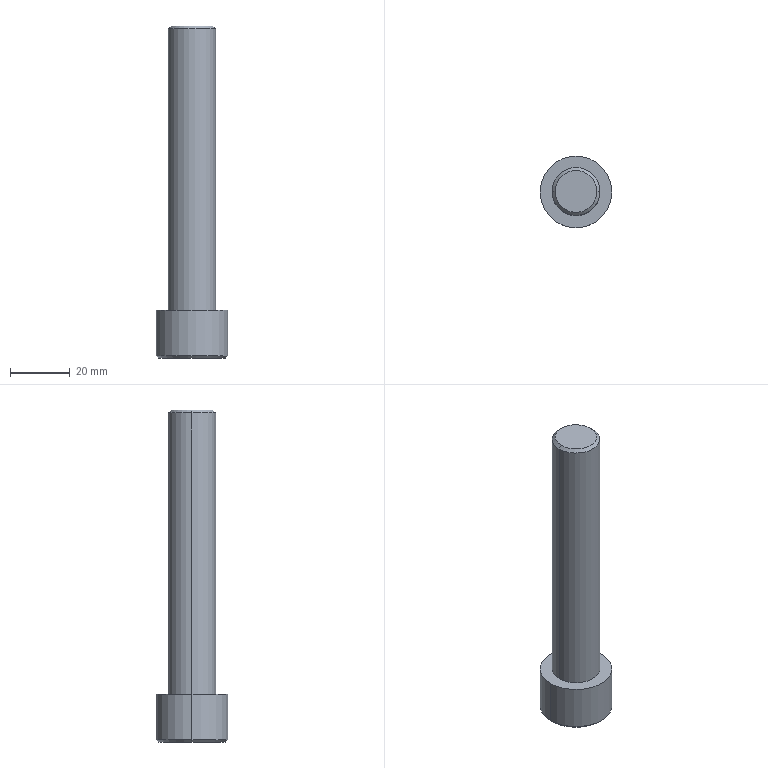Part | Creo | 1 solid | 18 faces | box 24 x 24 x 111 mm | volume 24662 mm3 | plane 10 | cylinder 4 | cone 4 | commonest cylinder face diameters 16 x2 24 x2
STEP:
#1=CARTESIAN_POINT('',(-139.,248.,-132.5));
#2=VERTEX_POINT('',#1);
#3=CARTESIAN_POINT('',(-115.,248.,-132.5));
#4=VERTEX_POINT('',#3);
#5=CARTESIAN_POINT('',(-127.,248.,-132.5));
#6=DIRECTION('',(0.,0.,1.));
#7=DIRECTION('',(-1.,0.,0.));
#8=AXIS2_PLACEMENT_3D('',#5,#6,#7);
#9=CIRCLE('',#8,12.);
#10=EDGE_CURVE('',#2,#4,#9,.T.);
#11=ORIENTED_EDGE('',*,*,#10,.F.);
#12=CARTESIAN_POINT('',(-127.,248.,-132.5));
#13=DIRECTION('',(0.,0.,1.));
#14=DIRECTION('',(1.,0.,0.));
#15=AXIS2_PLACEMENT_3D('',#12,#13,#14);
#16=CIRCLE('',#15,12.);
#17=EDGE_CURVE('',#4,#2,#16,.T.);
#18=ORIENTED_EDGE('',*,*,#17,.F.);
#19=EDGE_LOOP('',(#11,#18));
#20=FACE_OUTER_BOUND('',#19,.F.);
#21=CARTESIAN_POINT('',(-119.,248.,-132.5));
#22=VERTEX_POINT('',#21);
#23=CARTESIAN_POINT('',(-135.,248.,-132.5));
#24=VERTEX_POINT('',#23);
#25=CARTESIAN_POINT('',(-127.,248.,-132.5));
#26=DIRECTION('',(0.,0.,-1.));
#27=DIRECTION('',(1.,0.,0.));
#28=AXIS2_PLACEMENT_3D('',#25,#26,#27);
#29=CIRCLE('',#28,8.);
#30=EDGE_CURVE('',#22,#24,#29,.T.);
#31=ORIENTED_EDGE('',*,*,#30,.F.);
#32=CARTESIAN_POINT('',(-127.,248.,-132.5));
#33=DIRECTION('',(0.,0.,-1.));
#34=DIRECTION('',(-1.,0.,0.));
#35=AXIS2_PLACEMENT_3D('',#32,#33,#34);
#36=CIRCLE('',#35,8.);
#37=EDGE_CURVE('',#24,#22,#36,.T.);
#38=ORIENTED_EDGE('',*,*,#37,.F.);
#39=EDGE_LOOP('',(#31,#38));
#40=FACE_BOUND('',#39,.F.);
#41=CARTESIAN_POINT('',(-127.,248.,-132.5));
#42=DIRECTION('',(0.,0.,1.));
#43=DIRECTION('',(1.,0.,0.));
#44=AXIS2_PLACEMENT_3D('',#41,#42,#43);
#45=PLANE('',#44);
#46=ADVANCED_FACE('',(#20,#40),#45,.T.);
#47=CARTESIAN_POINT('',(-135.,248.,-38.5));
#48=VERTEX_POINT('',#47);
#49=CARTESIAN_POINT('',(-119.,248.,-38.5));
#50=VERTEX_POINT('',#49);
#51=CARTESIAN_POINT('',(-127.,248.,-38.5));
#52=DIRECTION('',(0.,0.,1.));
#53=DIRECTION('',(-1.,0.,0.));
#54=AXIS2_PLACEMENT_3D('',#51,#52,#53);
#55=CIRCLE('',#54,8.);
#56=EDGE_CURVE('',#48,#50,#55,.T.);
#57=ORIENTED_EDGE('',*,*,#56,.T.);
#58=CARTESIAN_POINT('',(-119.,248.,-132.5));
#59=DIRECTION('',(0.,0.,1.));
#60=VECTOR('',#59,94.);
#61=LINE('',#58,#60);
#62=EDGE_CURVE('',#22,#50,#61,.T.);
#63=ORIENTED_EDGE('',*,*,#62,.F.);
#64=ORIENTED_EDGE('',*,*,#30,.T.);
#65=CARTESIAN_POINT('',(-135.,248.,-132.5));
#66=DIRECTION('',(0.,0.,1.));
#67=VECTOR('',#66,94.);
#68=LINE('',#65,#67);
#69=EDGE_CURVE('',#24,#48,#68,.T.);
#70=ORIENTED_EDGE('',*,*,#69,.T.);
#71=EDGE_LOOP('',(#57,#63,#64,#70));
#72=FACE_OUTER_BOUND('',#71,.F.);
#73=CARTESIAN_POINT('',(-127.,248.,-150.5));
#74=DIRECTION('',(0.,0.,1.));
#75=DIRECTION('',(1.,0.,0.));
#76=AXIS2_PLACEMENT_3D('',#73,#74,#75);
#77=CYLINDRICAL_SURFACE('',#76,8.);
#78=ADVANCED_FACE('',(#72),#77,.T.);
#79=CARTESIAN_POINT('',(-134.,248.,-37.5));
#80=VERTEX_POINT('',#79);
#81=CARTESIAN_POINT('',(-120.,248.,-37.5));
#82=VERTEX_POINT('',#81);
#83=CARTESIAN_POINT('',(-127.,248.,-37.5));
#84=DIRECTION('',(0.,0.,1.));
#85=DIRECTION('',(-1.,0.,0.));
#86=AXIS2_PLACEMENT_3D('',#83,#84,#85);
#87=CIRCLE('',#86,7.);
#88=EDGE_CURVE('',#80,#82,#87,.T.);
#89=ORIENTED_EDGE('',*,*,#88,.T.);
#90=CARTESIAN_POINT('',(-120.,248.,-37.5));
#91=DIRECTION('',(0.7071,0.,-0.7071));
#92=VECTOR('',#91,1.414);
#93=LINE('',#90,#92);
#94=EDGE_CURVE('',#82,#50,#93,.T.);
#95=ORIENTED_EDGE('',*,*,#94,.T.);
#96=ORIENTED_EDGE('',*,*,#56,.F.);
#97=CARTESIAN_POINT('',(-134.,248.,-37.5));
#98=DIRECTION('',(-0.7071,0.,-0.7071));
#99=VECTOR('',#98,1.414);
#100=LINE('',#97,#99);
#101=EDGE_CURVE('',#80,#48,#100,.T.);
#102=ORIENTED_EDGE('',*,*,#101,.F.);
#103=EDGE_LOOP('',(#89,#95,#96,#102));
#104=FACE_OUTER_BOUND('',#103,.F.);
#105=CARTESIAN_POINT('',(-127.,248.,-38.));
#106=DIRECTION('',(0.,0.,-1.));
#107=DIRECTION('',(-1.,0.,0.));
#108=AXIS2_PLACEMENT_3D('',#105,#106,#107);
#109=CONICAL_SURFACE('',#108,7.5,45.);
#110=ADVANCED_FACE('',(#104),#109,.T.);
#111=CARTESIAN_POINT('',(-127.,248.,-37.5));
#112=DIRECTION('',(0.,0.,1.));
#113=DIRECTION('',(1.,0.,0.));
#114=AXIS2_PLACEMENT_3D('',#111,#112,#113);
#115=CIRCLE('',#114,7.);
#116=EDGE_CURVE('',#82,#80,#115,.T.);
#117=ORIENTED_EDGE('',*,*,#116,.F.);
#118=ORIENTED_EDGE('',*,*,#88,.F.);
#119=EDGE_LOOP('',(#117,#118));
#120=FACE_OUTER_BOUND('',#119,.F.);
#121=CARTESIAN_POINT('',(-127.,248.,-37.5));
#122=DIRECTION('',(0.,0.,1.));
#123=DIRECTION('',(1.,0.,0.));
#124=AXIS2_PLACEMENT_3D('',#121,#122,#123);
#125=PLANE('',#124);
#126=ADVANCED_FACE('',(#120),#125,.T.);
#127=ORIENTED_EDGE('',*,*,#116,.T.);
#128=ORIENTED_EDGE('',*,*,#101,.T.);
#129=CARTESIAN_POINT('',(-127.,248.,-38.5));
#130=DIRECTION('',(0.,0.,1.));
#131=DIRECTION('',(1.,0.,0.));
#132=AXIS2_PLACEMENT_3D('',#129,#130,#131);
#133=CIRCLE('',#132,8.);
#134=EDGE_CURVE('',#50,#48,#133,.T.);
#135=ORIENTED_EDGE('',*,*,#134,.F.);
#136=ORIENTED_EDGE('',*,*,#94,.F.);
#137=EDGE_LOOP('',(#127,#128,#135,#136));
#138=FACE_OUTER_BOUND('',#137,.F.);
#139=CARTESIAN_POINT('',(-127.,248.,-38.));
#140=DIRECTION('',(0.,0.,-1.));
#141=DIRECTION('',(-1.,0.,0.));
#142=AXIS2_PLACEMENT_3D('',#139,#140,#141);
#143=CONICAL_SURFACE('',#142,7.5,45.);
#144=ADVANCED_FACE('',(#138),#143,.T.);
#145=ORIENTED_EDGE('',*,*,#134,.T.);
#146=ORIENTED_EDGE('',*,*,#69,.F.);
#147=ORIENTED_EDGE('',*,*,#37,.T.);
#148=ORIENTED_EDGE('',*,*,#62,.T.);
#149=EDGE_LOOP('',(#145,#146,#147,#148));
#150=FACE_OUTER_BOUND('',#149,.F.);
#151=CARTESIAN_POINT('',(-127.,248.,-150.5));
#152=DIRECTION('',(0.,0.,1.));
#153=DIRECTION('',(1.,0.,0.));
#154=AXIS2_PLACEMENT_3D('',#151,#152,#153);
#155=CYLINDRICAL_SURFACE('',#154,8.);
#156=ADVANCED_FACE('',(#150),#155,.T.);
#157=CARTESIAN_POINT('',(-115.,248.,-147.7));
#158=VERTEX_POINT('',#157);
#159=CARTESIAN_POINT('',(-139.,248.,-147.7));
#160=VERTEX_POINT('',#159);
#161=CARTESIAN_POINT('',(-127.,248.,-147.7));
#162=DIRECTION('',(0.,0.,-1.));
#163=DIRECTION('',(1.,0.,0.));
#164=AXIS2_PLACEMENT_3D('',#161,#162,#163);
#165=CIRCLE('',#164,12.);
#166=EDGE_CURVE('',#158,#160,#165,.T.);
#167=ORIENTED_EDGE('',*,*,#166,.T.);
#168=CARTESIAN_POINT('',(-139.,248.,-147.7));
#169=DIRECTION('',(0.,0.,1.));
#170=VECTOR('',#169,15.2);
#171=LINE('',#168,#170);
#172=EDGE_CURVE('',#160,#2,#171,.T.);
#173=ORIENTED_EDGE('',*,*,#172,.T.);
#174=ORIENTED_EDGE('',*,*,#10,.T.);
#175=CARTESIAN_POINT('',(-115.,248.,-147.7));
#176=DIRECTION('',(0.,0.,1.));
#177=VECTOR('',#176,15.2);
#178=LINE('',#175,#177);
#179=EDGE_CURVE('',#158,#4,#178,.T.);
#180=ORIENTED_EDGE('',*,*,#179,.F.);
#181=EDGE_LOOP('',(#167,#173,#174,#180));
#182=FACE_OUTER_BOUND('',#181,.F.);
#183=CARTESIAN_POINT('',(-127.,248.,-150.5));
#184=DIRECTION('',(0.,0.,1.));
#185=DIRECTION('',(1.,0.,0.));
#186=AXIS2_PLACEMENT_3D('',#183,#184,#185);
#187=CYLINDRICAL_SURFACE('',#186,12.);
#188=ADVANCED_FACE('',(#182),#187,.T.);
#189=CARTESIAN_POINT('',(-115.8,248.,-148.5));
#190=VERTEX_POINT('',#189);
#191=CARTESIAN_POINT('',(-138.2,248.,-148.5));
#192=VERTEX_POINT('',#191);
#193=CARTESIAN_POINT('',(-127.,248.,-148.5));
#194=DIRECTION('',(0.,0.,-1.));
#195=DIRECTION('',(1.,0.,0.));
#196=AXIS2_PLACEMENT_3D('',#193,#194,#195);
#197=CIRCLE('',#196,11.2);
#198=EDGE_CURVE('',#190,#192,#197,.T.);
#199=ORIENTED_EDGE('',*,*,#198,.T.);
#200=CARTESIAN_POINT('',(-138.2,248.,-148.5));
#201=DIRECTION('',(-0.7071,0.,0.7071));
#202=VECTOR('',#201,1.131);
#203=LINE('',#200,#202);
#204=EDGE_CURVE('',#192,#160,#203,.T.);
#205=ORIENTED_EDGE('',*,*,#204,.T.);
#206=ORIENTED_EDGE('',*,*,#166,.F.);
#207=CARTESIAN_POINT('',(-115.8,248.,-148.5));
#208=DIRECTION('',(0.7071,0.,0.7071));
#209=VECTOR('',#208,1.131);
#210=LINE('',#207,#209);
#211=EDGE_CURVE('',#190,#158,#210,.T.);
#212=ORIENTED_EDGE('',*,*,#211,.F.);
#213=EDGE_LOOP('',(#199,#205,#206,#212));
#214=FACE_OUTER_BOUND('',#213,.F.);
#215=CARTESIAN_POINT('',(-127.,248.,-148.1));
#216=DIRECTION('',(0.,0.,1.));
#217=DIRECTION('',(1.,0.,0.));
#218=AXIS2_PLACEMENT_3D('',#215,#216,#217);
#219=CONICAL_SURFACE('',#218,11.6,45.);
#220=ADVANCED_FACE('',(#214),#219,.T.);
#221=ORIENTED_EDGE('',*,*,#198,.F.);
#222=CARTESIAN_POINT('',(-127.,248.,-148.5));
#223=DIRECTION('',(0.,0.,-1.));
#224=DIRECTION('',(-1.,0.,0.));
#225=AXIS2_PLACEMENT_3D('',#222,#223,#224);
#226=CIRCLE('',#225,11.2);
#227=EDGE_CURVE('',#192,#190,#226,.T.);
#228=ORIENTED_EDGE('',*,*,#227,.F.);
#229=EDGE_LOOP('',(#221,#228));
#230=FACE_OUTER_BOUND('',#229,.F.);
#231=CARTESIAN_POINT('',(-134.,243.959,-148.5));
#232=VERTEX_POINT('',#231);
#233=CARTESIAN_POINT('',(-127.,239.917,-148.5));
#234=VERTEX_POINT('',#233);
#235=CARTESIAN_POINT('',(-134.,243.959,-148.5));
#236=DIRECTION('',(0.866,-0.5,0.));
#237=VECTOR('',#236,8.083);
#238=LINE('',#235,#237);
#239=EDGE_CURVE('',#232,#234,#238,.T.);
#240=ORIENTED_EDGE('',*,*,#239,.F.);
#241=CARTESIAN_POINT('',(-134.,252.041,-148.5));
#242=VERTEX_POINT('',#241);
#243=CARTESIAN_POINT('',(-134.,252.041,-148.5));
#244=DIRECTION('',(0.,-1.,0.));
#245=VECTOR('',#244,8.083);
#246=LINE('',#243,#245);
#247=EDGE_CURVE('',#242,#232,#246,.T.);
#248=ORIENTED_EDGE('',*,*,#247,.F.);
#249=CARTESIAN_POINT('',(-127.,256.083,-148.5));
#250=VERTEX_POINT('',#249);
#251=CARTESIAN_POINT('',(-127.,256.083,-148.5));
#252=DIRECTION('',(-0.866,-0.5,0.));
#253=VECTOR('',#252,8.083);
#254=LINE('',#251,#253);
#255=EDGE_CURVE('',#250,#242,#254,.T.);
#256=ORIENTED_EDGE('',*,*,#255,.F.);
#257=CARTESIAN_POINT('',(-120.,252.041,-148.5));
#258=VERTEX_POINT('',#257);
#259=CARTESIAN_POINT('',(-120.,252.041,-148.5));
#260=DIRECTION('',(-0.866,0.5,0.));
#261=VECTOR('',#260,8.083);
#262=LINE('',#259,#261);
#263=EDGE_CURVE('',#258,#250,#262,.T.);
#264=ORIENTED_EDGE('',*,*,#263,.F.);
#265=CARTESIAN_POINT('',(-120.,243.959,-148.5));
#266=VERTEX_POINT('',#265);
#267=CARTESIAN_POINT('',(-120.,243.959,-148.5));
#268=DIRECTION('',(0.,1.,0.));
#269=VECTOR('',#268,8.083);
#270=LINE('',#267,#269);
#271=EDGE_CURVE('',#266,#258,#270,.T.);
#272=ORIENTED_EDGE('',*,*,#271,.F.);
#273=CARTESIAN_POINT('',(-127.,239.917,-148.5));
#274=DIRECTION('',(0.866,0.5,0.));
#275=VECTOR('',#274,8.083);
#276=LINE('',#273,#275);
#277=EDGE_CURVE('',#234,#266,#276,.T.);
#278=ORIENTED_EDGE('',*,*,#277,.F.);
#279=EDGE_LOOP('',(#240,#248,#256,#264,#272,#278));
#280=FACE_BOUND('',#279,.F.);
#281=CARTESIAN_POINT('',(-127.,248.,-148.5));
#282=DIRECTION('',(0.,0.,1.));
#283=DIRECTION('',(1.,0.,0.));
#284=AXIS2_PLACEMENT_3D('',#281,#282,#283);
#285=PLANE('',#284);
#286=ADVANCED_FACE('',(#230,#280),#285,.F.);
#287=ORIENTED_EDGE('',*,*,#227,.T.);
#288=ORIENTED_EDGE('',*,*,#211,.T.);
#289=CARTESIAN_POINT('',(-127.,248.,-147.7));
#290=DIRECTION('',(0.,0.,-1.));
#291=DIRECTION('',(-1.,0.,0.));
#292=AXIS2_PLACEMENT_3D('',#289,#290,#291);
#293=CIRCLE('',#292,12.);
#294=EDGE_CURVE('',#160,#158,#293,.T.);
#295=ORIENTED_EDGE('',*,*,#294,.F.);
#296=ORIENTED_EDGE('',*,*,#204,.F.);
#297=EDGE_LOOP('',(#287,#288,#295,#296));
#298=FACE_OUTER_BOUND('',#297,.F.);
#299=CARTESIAN_POINT('',(-127.,248.,-148.1));
#300=DIRECTION('',(0.,0.,1.));
#301=DIRECTION('',(1.,0.,0.));
#302=AXIS2_PLACEMENT_3D('',#299,#300,#301);
#303=CONICAL_SURFACE('',#302,11.6,45.);
#304=ADVANCED_FACE('',(#298),#303,.T.);
#305=ORIENTED_EDGE('',*,*,#294,.T.);
#306=ORIENTED_EDGE('',*,*,#179,.T.);
#307=ORIENTED_EDGE('',*,*,#17,.T.);
#308=ORIENTED_EDGE('',*,*,#172,.F.);
#309=EDGE_LOOP('',(#305,#306,#307,#308));
#310=FACE_OUTER_BOUND('',#309,.F.);
#311=CARTESIAN_POINT('',(-127.,248.,-150.5));
#312=DIRECTION('',(0.,0.,1.));
#313=DIRECTION('',(1.,0.,0.));
#314=AXIS2_PLACEMENT_3D('',#311,#312,#313);
#315=CYLINDRICAL_SURFACE('',#314,12.);
#316=ADVANCED_FACE('',(#310),#315,.T.);
#317=ORIENTED_EDGE('',*,*,#239,.T.);
#318=CARTESIAN_POINT('',(-127.,239.917,-138.9));
#319=VERTEX_POINT('',#318);
#320=CARTESIAN_POINT('',(-127.,239.917,-148.5));
#321=DIRECTION('',(0.,0.,1.));
#322=VECTOR('',#321,9.6);
#323=LINE('',#320,#322);
#324=EDGE_CURVE('',#234,#319,#323,.T.);
#325=ORIENTED_EDGE('',*,*,#324,.T.);
#326=CARTESIAN_POINT('',(-134.,243.959,-138.9));
#327=VERTEX_POINT('',#326);
#328=CARTESIAN_POINT('',(-127.,239.917,-138.9));
#329=DIRECTION('',(-0.866,0.5,0.));
#330=VECTOR('',#329,8.083);
#331=LINE('',#328,#330);
#332=EDGE_CURVE('',#319,#327,#331,.T.);
#333=ORIENTED_EDGE('',*,*,#332,.T.);
#334=CARTESIAN_POINT('',(-134.,243.959,-148.5));
#335=DIRECTION('',(0.,0.,1.));
#336=VECTOR('',#335,9.6);
#337=LINE('',#334,#336);
#338=EDGE_CURVE('',#232,#327,#337,.T.);
#339=ORIENTED_EDGE('',*,*,#338,.F.);
#340=EDGE_LOOP('',(#317,#325,#333,#339));
#341=FACE_OUTER_BOUND('',#340,.F.);
#342=CARTESIAN_POINT('',(-127.,239.917,-138.9));
#343=DIRECTION('',(-0.5,-0.866,0.));
#344=DIRECTION('',(0.866,-0.5,0.));
#345=AXIS2_PLACEMENT_3D('',#342,#343,#344);
#346=PLANE('',#345);
#347=ADVANCED_FACE('',(#341),#346,.F.);
#348=ORIENTED_EDGE('',*,*,#277,.T.);
#349=CARTESIAN_POINT('',(-120.,243.959,-138.9));
#350=VERTEX_POINT('',#349);
#351=CARTESIAN_POINT('',(-120.,243.959,-148.5));
#352=DIRECTION('',(0.,0.,1.));
#353=VECTOR('',#352,9.6);
#354=LINE('',#351,#353);
#355=EDGE_CURVE('',#266,#350,#354,.T.);
#356=ORIENTED_EDGE('',*,*,#355,.T.);
#357=CARTESIAN_POINT('',(-120.,243.959,-138.9));
#358=DIRECTION('',(-0.866,-0.5,0.));
#359=VECTOR('',#358,8.083);
#360=LINE('',#357,#359);
#361=EDGE_CURVE('',#350,#319,#360,.T.);
#362=ORIENTED_EDGE('',*,*,#361,.T.);
#363=ORIENTED_EDGE('',*,*,#324,.F.);
#364=EDGE_LOOP('',(#348,#356,#362,#363));
#365=FACE_OUTER_BOUND('',#364,.F.);
#366=CARTESIAN_POINT('',(-120.,243.959,-138.9));
#367=DIRECTION('',(0.5,-0.866,0.));
#368=DIRECTION('',(0.866,0.5,0.));
#369=AXIS2_PLACEMENT_3D('',#366,#367,#368);
#370=PLANE('',#369);
#371=ADVANCED_FACE('',(#365),#370,.F.);
#372=ORIENTED_EDGE('',*,*,#271,.T.);
#373=CARTESIAN_POINT('',(-120.,252.041,-138.9));
#374=VERTEX_POINT('',#373);
#375=CARTESIAN_POINT('',(-120.,252.041,-148.5));
#376=DIRECTION('',(0.,0.,1.));
#377=VECTOR('',#376,9.6);
#378=LINE('',#375,#377);
#379=EDGE_CURVE('',#258,#374,#378,.T.);
#380=ORIENTED_EDGE('',*,*,#379,.T.);
#381=CARTESIAN_POINT('',(-120.,243.959,-138.9));
#382=DIRECTION('',(0.,1.,0.));
#383=VECTOR('',#382,8.083);
#384=LINE('',#381,#383);
#385=EDGE_CURVE('',#350,#374,#384,.T.);
#386=ORIENTED_EDGE('',*,*,#385,.F.);
#387=ORIENTED_EDGE('',*,*,#355,.F.);
#388=EDGE_LOOP('',(#372,#380,#386,#387));
#389=FACE_OUTER_BOUND('',#388,.F.);
#390=CARTESIAN_POINT('',(-120.,252.041,-138.9));
#391=DIRECTION('',(1.,0.,0.));
#392=DIRECTION('',(0.,0.,-1.));
#393=AXIS2_PLACEMENT_3D('',#390,#391,#392);
#394=PLANE('',#393);
#395=ADVANCED_FACE('',(#389),#394,.F.);
#396=ORIENTED_EDGE('',*,*,#263,.T.);
#397=CARTESIAN_POINT('',(-127.,256.083,-138.9));
#398=VERTEX_POINT('',#397);
#399=CARTESIAN_POINT('',(-127.,256.083,-148.5));
#400=DIRECTION('',(0.,0.,1.));
#401=VECTOR('',#400,9.6);
#402=LINE('',#399,#401);
#403=EDGE_CURVE('',#250,#398,#402,.T.);
#404=ORIENTED_EDGE('',*,*,#403,.T.);
#405=CARTESIAN_POINT('',(-127.,256.083,-138.9));
#406=DIRECTION('',(0.866,-0.5,0.));
#407=VECTOR('',#406,8.083);
#408=LINE('',#405,#407);
#409=EDGE_CURVE('',#398,#374,#408,.T.);
#410=ORIENTED_EDGE('',*,*,#409,.T.);
#411=ORIENTED_EDGE('',*,*,#379,.F.);
#412=EDGE_LOOP('',(#396,#404,#410,#411));
#413=FACE_OUTER_BOUND('',#412,.F.);
#414=CARTESIAN_POINT('',(-127.,256.083,-138.9));
#415=DIRECTION('',(0.5,0.866,0.));
#416=DIRECTION('',(-0.866,0.5,0.));
#417=AXIS2_PLACEMENT_3D('',#414,#415,#416);
#418=PLANE('',#417);
#419=ADVANCED_FACE('',(#413),#418,.F.);
#420=ORIENTED_EDGE('',*,*,#255,.T.);
#421=CARTESIAN_POINT('',(-134.,252.041,-138.9));
#422=VERTEX_POINT('',#421);
#423=CARTESIAN_POINT('',(-134.,252.041,-148.5));
#424=DIRECTION('',(0.,0.,1.));
#425=VECTOR('',#424,9.6);
#426=LINE('',#423,#425);
#427=EDGE_CURVE('',#242,#422,#426,.T.);
#428=ORIENTED_EDGE('',*,*,#427,.T.);
#429=CARTESIAN_POINT('',(-134.,252.041,-138.9));
#430=DIRECTION('',(0.866,0.5,0.));
#431=VECTOR('',#430,8.083);
#432=LINE('',#429,#431);
#433=EDGE_CURVE('',#422,#398,#432,.T.);
#434=ORIENTED_EDGE('',*,*,#433,.T.);
#435=ORIENTED_EDGE('',*,*,#403,.F.);
#436=EDGE_LOOP('',(#420,#428,#434,#435));
#437=FACE_OUTER_BOUND('',#436,.F.);
#438=CARTESIAN_POINT('',(-134.,252.041,-138.9));
#439=DIRECTION('',(-0.5,0.866,0.));
#440=DIRECTION('',(-0.866,-0.5,0.));
#441=AXIS2_PLACEMENT_3D('',#438,#439,#440);
#442=PLANE('',#441);
#443=ADVANCED_FACE('',(#437),#442,.F.);
#444=ORIENTED_EDGE('',*,*,#247,.T.);
#445=ORIENTED_EDGE('',*,*,#338,.T.);
#446=CARTESIAN_POINT('',(-134.,252.041,-138.9));
#447=DIRECTION('',(0.,-1.,0.));
#448=VECTOR('',#447,8.083);
#449=LINE('',#446,#448);
#450=EDGE_CURVE('',#422,#327,#449,.T.);
#451=ORIENTED_EDGE('',*,*,#450,.F.);
#452=ORIENTED_EDGE('',*,*,#427,.F.);
#453=EDGE_LOOP('',(#444,#445,#451,#452));
#454=FACE_OUTER_BOUND('',#453,.F.);
#455=CARTESIAN_POINT('',(-134.,243.959,-138.9));
#456=DIRECTION('',(-1.,0.,0.));
#457=DIRECTION('',(0.,0.,1.));
#458=AXIS2_PLACEMENT_3D('',#455,#456,#457);
#459=PLANE('',#458);
#460=ADVANCED_FACE('',(#454),#459,.F.);
#461=ORIENTED_EDGE('',*,*,#361,.F.);
#462=ORIENTED_EDGE('',*,*,#385,.T.);
#463=ORIENTED_EDGE('',*,*,#409,.F.);
#464=ORIENTED_EDGE('',*,*,#433,.F.);
#465=ORIENTED_EDGE('',*,*,#450,.T.);
#466=ORIENTED_EDGE('',*,*,#332,.F.);
#467=EDGE_LOOP('',(#461,#462,#463,#464,#465,#466));
#468=FACE_OUTER_BOUND('',#467,.F.);
#469=CARTESIAN_POINT('',(-113.,248.,-138.9));
#470=DIRECTION('',(0.,0.,1.));
#471=DIRECTION('',(1.,0.,0.));
#472=AXIS2_PLACEMENT_3D('',#469,#470,#471);
#473=PLANE('',#472);
#474=ADVANCED_FACE('',(#468),#473,.F.);
#475=CLOSED_SHELL('',(#46,#78,#110,#126,#144,#156,#188,#220,#286,#304,#316,#347,#371,#395,#419,#443,#460,#474));
#476=MANIFOLD_SOLID_BREP('',#475);
#477=(LENGTH_UNIT()NAMED_UNIT(*)SI_UNIT(.MILLI.,.METRE.));
#478=UNCERTAINTY_MEASURE_WITH_UNIT(LENGTH_MEASURE(0.01161),#477,'','');
#479=(NAMED_UNIT(*)PLANE_ANGLE_UNIT()SI_UNIT($,.RADIAN.));
#480=PLANE_ANGLE_MEASURE_WITH_UNIT(PLANE_ANGLE_MEASURE(0.01745),#479);
#481=(CONVERSION_BASED_UNIT('DEGREE',#480)NAMED_UNIT(*)PLANE_ANGLE_UNIT());
#482=(NAMED_UNIT(*)SI_UNIT($,.STERADIAN.)SOLID_ANGLE_UNIT());
#483=(GEOMETRIC_REPRESENTATION_CONTEXT(3)GLOBAL_UNCERTAINTY_ASSIGNED_CONTEXT((#478))GLOBAL_UNIT_ASSIGNED_CONTEXT((#477,#481,#482))REPRESENTATION_CONTEXT('',''));
#484=ADVANCED_BREP_SHAPE_REPRESENTATION('',(#476),#483);